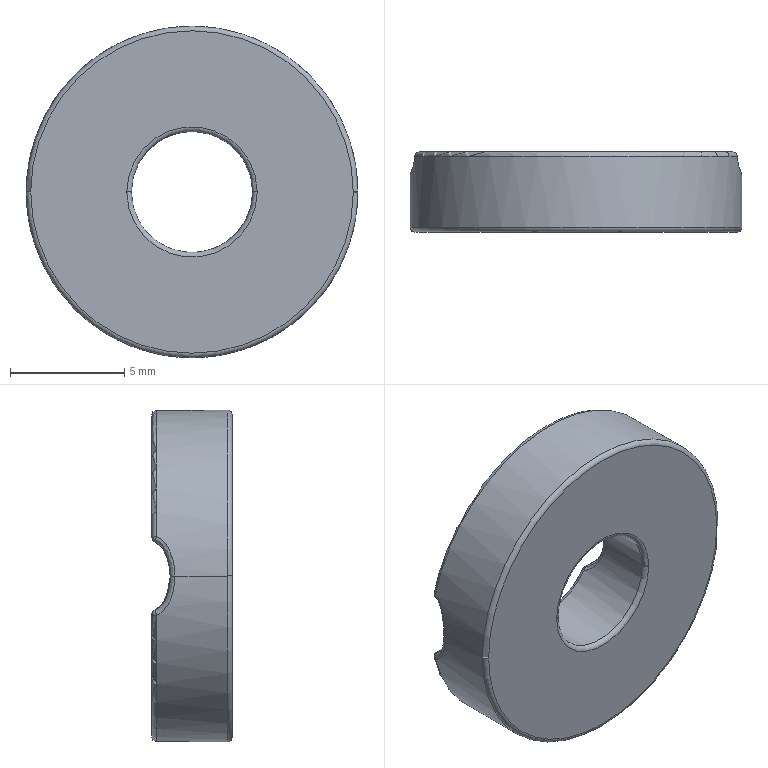Part | STEP file | ZITUIZHOUCHEN2_3_1_2_1_1 | 1 solid | 37 faces | box 14.5 x 3.5 x 14.5 mm | volume 481.95 mm3 | torus 8 | cylinder 8 | spline 8 | sphere 8 | plane 3 | other 2 | commonest cylinder face diameters 0.4 x4 5.3 x2 14.5 x2